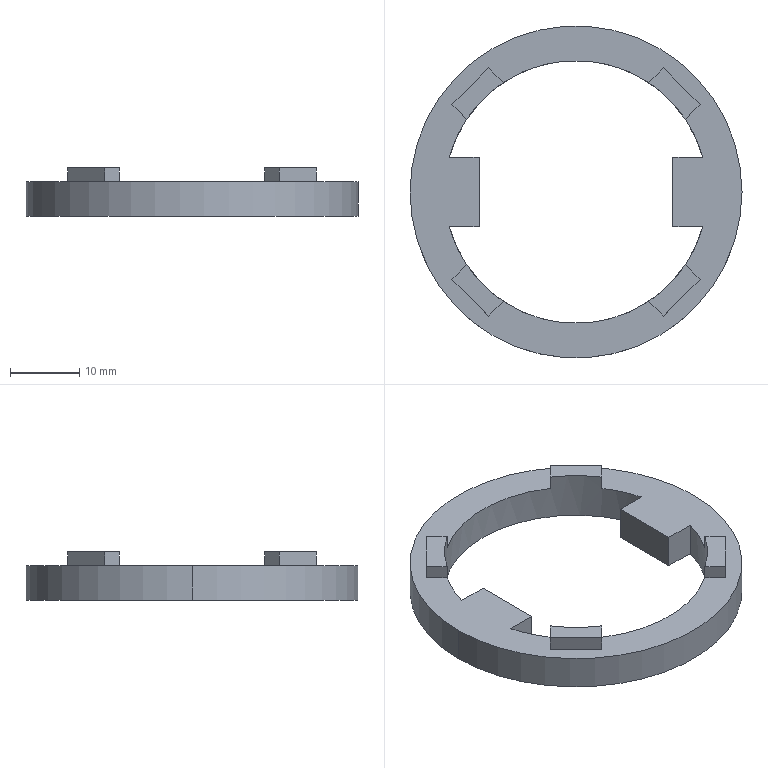Part | SolidWorks | features Extrusion 1, ICE 1 | 1 solid | 28 faces | box 48 x 48 x 7 mm | volume 4020 mm3 | plane 24 | cylinder 4 | commonest cylinder face diameters 38 x2 48 x2
STEP:
#1=CARTESIAN_POINT('',(24.,0.,5.));
#2=VERTEX_POINT('',#1);
#3=CARTESIAN_POINT('',(-24.,0.,5.));
#4=VERTEX_POINT('',#3);
#5=CARTESIAN_POINT('',(0.,0.,5.));
#6=DIRECTION('',(0.,0.,1.));
#7=DIRECTION('',(1.,0.,0.));
#8=AXIS2_PLACEMENT_3D('',#5,#6,#7);
#9=CIRCLE('',#8,24.);
#10=EDGE_CURVE('',#2,#4,#9,.T.);
#11=ORIENTED_EDGE('',*,*,#10,.F.);
#12=CARTESIAN_POINT('',(24.,0.,0.));
#13=VERTEX_POINT('',#12);
#14=CARTESIAN_POINT('',(24.,0.,5.));
#15=DIRECTION('',(0.,0.,-1.));
#16=VECTOR('',#15,1000.);
#17=LINE('',#14,#16);
#18=EDGE_CURVE('',#2,#13,#17,.T.);
#19=ORIENTED_EDGE('',*,*,#18,.T.);
#20=CARTESIAN_POINT('',(-24.,0.,0.));
#21=VERTEX_POINT('',#20);
#22=CARTESIAN_POINT('',(0.,0.,0.));
#23=DIRECTION('',(0.,0.,1.));
#24=DIRECTION('',(1.,0.,0.));
#25=AXIS2_PLACEMENT_3D('',#22,#23,#24);
#26=CIRCLE('',#25,24.);
#27=EDGE_CURVE('',#13,#21,#26,.T.);
#28=ORIENTED_EDGE('',*,*,#27,.T.);
#29=CARTESIAN_POINT('',(-24.,0.,5.));
#30=DIRECTION('',(0.,0.,-1.));
#31=VECTOR('',#30,1000.);
#32=LINE('',#29,#31);
#33=EDGE_CURVE('',#4,#21,#32,.T.);
#34=ORIENTED_EDGE('',*,*,#33,.F.);
#35=EDGE_LOOP('',(#11,#19,#28,#34));
#36=FACE_OUTER_BOUND('',#35,.T.);
#37=CARTESIAN_POINT('',(0.,0.,5.));
#38=DIRECTION('',(0.,0.,-1.));
#39=DIRECTION('',(-1.,0.,0.));
#40=AXIS2_PLACEMENT_3D('',#37,#38,#39);
#41=CYLINDRICAL_SURFACE('',#40,24.);
#42=ADVANCED_FACE('',(#36),#41,.T.);
#43=CARTESIAN_POINT('',(0.,0.,5.));
#44=DIRECTION('',(0.,0.,1.));
#45=DIRECTION('',(1.,0.,0.));
#46=AXIS2_PLACEMENT_3D('',#43,#44,#45);
#47=CIRCLE('',#46,24.);
#48=EDGE_CURVE('',#4,#2,#47,.T.);
#49=ORIENTED_EDGE('',*,*,#48,.T.);
#50=ORIENTED_EDGE('',*,*,#10,.T.);
#51=EDGE_LOOP('',(#49,#50));
#52=FACE_OUTER_BOUND('',#51,.T.);
#53=CARTESIAN_POINT('',(-17.944,-12.64,5.));
#54=VERTEX_POINT('',#53);
#55=CARTESIAN_POINT('',(-12.64,-17.944,5.));
#56=VERTEX_POINT('',#55);
#57=CARTESIAN_POINT('',(-12.64,-17.944,5.));
#58=DIRECTION('',(0.7071,-0.7071,0.));
#59=VECTOR('',#58,1000.);
#60=LINE('',#57,#59);
#61=EDGE_CURVE('',#54,#56,#60,.T.);
#62=ORIENTED_EDGE('',*,*,#61,.F.);
#63=CARTESIAN_POINT('',(-15.822,-10.519,5.));
#64=VERTEX_POINT('',#63);
#65=CARTESIAN_POINT('',(-15.822,-10.519,5.));
#66=DIRECTION('',(-0.7071,-0.7071,0.));
#67=VECTOR('',#66,1000.);
#68=LINE('',#65,#67);
#69=EDGE_CURVE('',#64,#54,#68,.T.);
#70=ORIENTED_EDGE('',*,*,#69,.F.);
#71=CARTESIAN_POINT('',(-18.33,-5.,5.));
#72=VERTEX_POINT('',#71);
#73=CARTESIAN_POINT('',(0.,0.,5.));
#74=DIRECTION('',(0.,0.,1.));
#75=DIRECTION('',(1.,0.,0.));
#76=AXIS2_PLACEMENT_3D('',#73,#74,#75);
#77=CIRCLE('',#76,19.);
#78=EDGE_CURVE('',#72,#64,#77,.T.);
#79=ORIENTED_EDGE('',*,*,#78,.F.);
#80=CARTESIAN_POINT('',(-14.,-5.,5.));
#81=VERTEX_POINT('',#80);
#82=CARTESIAN_POINT('',(-18.33,-5.,5.));
#83=DIRECTION('',(-1.,0.,0.));
#84=VECTOR('',#83,1000.);
#85=LINE('',#82,#84);
#86=EDGE_CURVE('',#81,#72,#85,.T.);
#87=ORIENTED_EDGE('',*,*,#86,.F.);
#88=CARTESIAN_POINT('',(-14.,5.,5.));
#89=VERTEX_POINT('',#88);
#90=CARTESIAN_POINT('',(-14.,5.,5.));
#91=DIRECTION('',(0.,-1.,0.));
#92=VECTOR('',#91,1000.);
#93=LINE('',#90,#92);
#94=EDGE_CURVE('',#89,#81,#93,.T.);
#95=ORIENTED_EDGE('',*,*,#94,.F.);
#96=CARTESIAN_POINT('',(-18.33,5.,5.));
#97=VERTEX_POINT('',#96);
#98=CARTESIAN_POINT('',(-18.33,5.,5.));
#99=DIRECTION('',(1.,0.,0.));
#100=VECTOR('',#99,1000.);
#101=LINE('',#98,#100);
#102=EDGE_CURVE('',#97,#89,#101,.T.);
#103=ORIENTED_EDGE('',*,*,#102,.F.);
#104=CARTESIAN_POINT('',(-15.822,10.519,5.));
#105=VERTEX_POINT('',#104);
#106=CARTESIAN_POINT('',(0.,0.,5.));
#107=DIRECTION('',(0.,0.,1.));
#108=DIRECTION('',(1.,0.,0.));
#109=AXIS2_PLACEMENT_3D('',#106,#107,#108);
#110=CIRCLE('',#109,19.);
#111=EDGE_CURVE('',#105,#97,#110,.T.);
#112=ORIENTED_EDGE('',*,*,#111,.F.);
#113=CARTESIAN_POINT('',(-17.944,12.64,5.));
#114=VERTEX_POINT('',#113);
#115=CARTESIAN_POINT('',(-15.822,10.519,5.));
#116=DIRECTION('',(0.7071,-0.7071,0.));
#117=VECTOR('',#116,1000.);
#118=LINE('',#115,#117);
#119=EDGE_CURVE('',#114,#105,#118,.T.);
#120=ORIENTED_EDGE('',*,*,#119,.F.);
#121=CARTESIAN_POINT('',(-12.64,17.944,5.));
#122=VERTEX_POINT('',#121);
#123=CARTESIAN_POINT('',(-17.944,12.64,5.));
#124=DIRECTION('',(-0.7071,-0.7071,0.));
#125=VECTOR('',#124,1000.);
#126=LINE('',#123,#125);
#127=EDGE_CURVE('',#122,#114,#126,.T.);
#128=ORIENTED_EDGE('',*,*,#127,.F.);
#129=CARTESIAN_POINT('',(-10.519,15.822,5.));
#130=VERTEX_POINT('',#129);
#131=CARTESIAN_POINT('',(-10.519,15.822,5.));
#132=DIRECTION('',(-0.7071,0.7071,0.));
#133=VECTOR('',#132,1000.);
#134=LINE('',#131,#133);
#135=EDGE_CURVE('',#130,#122,#134,.T.);
#136=ORIENTED_EDGE('',*,*,#135,.F.);
#137=CARTESIAN_POINT('',(10.519,15.822,5.));
#138=VERTEX_POINT('',#137);
#139=CARTESIAN_POINT('',(0.,0.,5.));
#140=DIRECTION('',(0.,0.,1.));
#141=DIRECTION('',(1.,0.,0.));
#142=AXIS2_PLACEMENT_3D('',#139,#140,#141);
#143=CIRCLE('',#142,19.);
#144=EDGE_CURVE('',#138,#130,#143,.T.);
#145=ORIENTED_EDGE('',*,*,#144,.F.);
#146=CARTESIAN_POINT('',(12.64,17.944,5.));
#147=VERTEX_POINT('',#146);
#148=CARTESIAN_POINT('',(10.519,15.822,5.));
#149=DIRECTION('',(-0.7071,-0.7071,0.));
#150=VECTOR('',#149,1000.);
#151=LINE('',#148,#150);
#152=EDGE_CURVE('',#147,#138,#151,.T.);
#153=ORIENTED_EDGE('',*,*,#152,.F.);
#154=CARTESIAN_POINT('',(17.944,12.64,5.));
#155=VERTEX_POINT('',#154);
#156=CARTESIAN_POINT('',(12.64,17.944,5.));
#157=DIRECTION('',(-0.7071,0.7071,0.));
#158=VECTOR('',#157,1000.);
#159=LINE('',#156,#158);
#160=EDGE_CURVE('',#155,#147,#159,.T.);
#161=ORIENTED_EDGE('',*,*,#160,.F.);
#162=CARTESIAN_POINT('',(15.822,10.519,5.));
#163=VERTEX_POINT('',#162);
#164=CARTESIAN_POINT('',(15.822,10.519,5.));
#165=DIRECTION('',(0.7071,0.7071,0.));
#166=VECTOR('',#165,1000.);
#167=LINE('',#164,#166);
#168=EDGE_CURVE('',#163,#155,#167,.T.);
#169=ORIENTED_EDGE('',*,*,#168,.F.);
#170=CARTESIAN_POINT('',(18.33,5.,5.));
#171=VERTEX_POINT('',#170);
#172=CARTESIAN_POINT('',(0.,0.,5.));
#173=DIRECTION('',(0.,0.,1.));
#174=DIRECTION('',(1.,0.,0.));
#175=AXIS2_PLACEMENT_3D('',#172,#173,#174);
#176=CIRCLE('',#175,19.);
#177=EDGE_CURVE('',#171,#163,#176,.T.);
#178=ORIENTED_EDGE('',*,*,#177,.F.);
#179=CARTESIAN_POINT('',(14.,5.,5.));
#180=VERTEX_POINT('',#179);
#181=CARTESIAN_POINT('',(18.33,5.,5.));
#182=DIRECTION('',(1.,0.,0.));
#183=VECTOR('',#182,1000.);
#184=LINE('',#181,#183);
#185=EDGE_CURVE('',#180,#171,#184,.T.);
#186=ORIENTED_EDGE('',*,*,#185,.F.);
#187=CARTESIAN_POINT('',(14.,-5.,5.));
#188=VERTEX_POINT('',#187);
#189=CARTESIAN_POINT('',(14.,5.,5.));
#190=DIRECTION('',(0.,1.,0.));
#191=VECTOR('',#190,1000.);
#192=LINE('',#189,#191);
#193=EDGE_CURVE('',#188,#180,#192,.T.);
#194=ORIENTED_EDGE('',*,*,#193,.F.);
#195=CARTESIAN_POINT('',(18.33,-5.,5.));
#196=VERTEX_POINT('',#195);
#197=CARTESIAN_POINT('',(18.33,-5.,5.));
#198=DIRECTION('',(-1.,0.,0.));
#199=VECTOR('',#198,1000.);
#200=LINE('',#197,#199);
#201=EDGE_CURVE('',#196,#188,#200,.T.);
#202=ORIENTED_EDGE('',*,*,#201,.F.);
#203=CARTESIAN_POINT('',(15.822,-10.519,5.));
#204=VERTEX_POINT('',#203);
#205=CARTESIAN_POINT('',(0.,0.,5.));
#206=DIRECTION('',(0.,0.,1.));
#207=DIRECTION('',(1.,0.,0.));
#208=AXIS2_PLACEMENT_3D('',#205,#206,#207);
#209=CIRCLE('',#208,19.);
#210=EDGE_CURVE('',#204,#196,#209,.T.);
#211=ORIENTED_EDGE('',*,*,#210,.F.);
#212=CARTESIAN_POINT('',(17.944,-12.64,5.));
#213=VERTEX_POINT('',#212);
#214=CARTESIAN_POINT('',(15.822,-10.519,5.));
#215=DIRECTION('',(-0.7071,0.7071,0.));
#216=VECTOR('',#215,1000.);
#217=LINE('',#214,#216);
#218=EDGE_CURVE('',#213,#204,#217,.T.);
#219=ORIENTED_EDGE('',*,*,#218,.F.);
#220=CARTESIAN_POINT('',(12.64,-17.944,5.));
#221=VERTEX_POINT('',#220);
#222=CARTESIAN_POINT('',(17.944,-12.64,5.));
#223=DIRECTION('',(0.7071,0.7071,0.));
#224=VECTOR('',#223,1000.);
#225=LINE('',#222,#224);
#226=EDGE_CURVE('',#221,#213,#225,.T.);
#227=ORIENTED_EDGE('',*,*,#226,.F.);
#228=CARTESIAN_POINT('',(10.519,-15.822,5.));
#229=VERTEX_POINT('',#228);
#230=CARTESIAN_POINT('',(10.519,-15.822,5.));
#231=DIRECTION('',(0.7071,-0.7071,0.));
#232=VECTOR('',#231,1000.);
#233=LINE('',#230,#232);
#234=EDGE_CURVE('',#229,#221,#233,.T.);
#235=ORIENTED_EDGE('',*,*,#234,.F.);
#236=CARTESIAN_POINT('',(-10.519,-15.822,5.));
#237=VERTEX_POINT('',#236);
#238=CARTESIAN_POINT('',(0.,0.,5.));
#239=DIRECTION('',(0.,0.,1.));
#240=DIRECTION('',(1.,0.,0.));
#241=AXIS2_PLACEMENT_3D('',#238,#239,#240);
#242=CIRCLE('',#241,19.);
#243=EDGE_CURVE('',#237,#229,#242,.T.);
#244=ORIENTED_EDGE('',*,*,#243,.F.);
#245=CARTESIAN_POINT('',(-10.519,-15.822,5.));
#246=DIRECTION('',(0.7071,0.7071,0.));
#247=VECTOR('',#246,1000.);
#248=LINE('',#245,#247);
#249=EDGE_CURVE('',#56,#237,#248,.T.);
#250=ORIENTED_EDGE('',*,*,#249,.F.);
#251=EDGE_LOOP('',(#62,#70,#79,#87,#95,#103,#112,#120,#128,#136,#145,#153,#161,#169,#178,#186,#194,#202,#211,#219,#227,#235,#244,#250));
#252=FACE_BOUND('',#251,.T.);
#253=CARTESIAN_POINT('',(0.,0.,5.));
#254=DIRECTION('',(0.,0.,1.));
#255=DIRECTION('',(1.,0.,0.));
#256=AXIS2_PLACEMENT_3D('',#253,#254,#255);
#257=PLANE('',#256);
#258=ADVANCED_FACE('',(#52,#252),#257,.T.);
#259=CARTESIAN_POINT('',(0.,0.,0.));
#260=DIRECTION('',(0.,0.,1.));
#261=DIRECTION('',(1.,0.,0.));
#262=AXIS2_PLACEMENT_3D('',#259,#260,#261);
#263=CIRCLE('',#262,24.);
#264=EDGE_CURVE('',#21,#13,#263,.T.);
#265=ORIENTED_EDGE('',*,*,#264,.F.);
#266=ORIENTED_EDGE('',*,*,#27,.F.);
#267=EDGE_LOOP('',(#265,#266));
#268=FACE_OUTER_BOUND('',#267,.T.);
#269=CARTESIAN_POINT('',(18.33,5.,0.));
#270=VERTEX_POINT('',#269);
#271=CARTESIAN_POINT('',(-18.33,5.,0.));
#272=VERTEX_POINT('',#271);
#273=CARTESIAN_POINT('',(0.,0.,0.));
#274=DIRECTION('',(0.,0.,1.));
#275=DIRECTION('',(1.,0.,0.));
#276=AXIS2_PLACEMENT_3D('',#273,#274,#275);
#277=CIRCLE('',#276,19.);
#278=EDGE_CURVE('',#270,#272,#277,.T.);
#279=ORIENTED_EDGE('',*,*,#278,.T.);
#280=CARTESIAN_POINT('',(-14.,5.,0.));
#281=VERTEX_POINT('',#280);
#282=CARTESIAN_POINT('',(-18.33,5.,0.));
#283=DIRECTION('',(1.,0.,0.));
#284=VECTOR('',#283,1000.);
#285=LINE('',#282,#284);
#286=EDGE_CURVE('',#272,#281,#285,.T.);
#287=ORIENTED_EDGE('',*,*,#286,.T.);
#288=CARTESIAN_POINT('',(-14.,-5.,0.));
#289=VERTEX_POINT('',#288);
#290=CARTESIAN_POINT('',(-14.,5.,0.));
#291=DIRECTION('',(0.,-1.,0.));
#292=VECTOR('',#291,1000.);
#293=LINE('',#290,#292);
#294=EDGE_CURVE('',#281,#289,#293,.T.);
#295=ORIENTED_EDGE('',*,*,#294,.T.);
#296=CARTESIAN_POINT('',(-18.33,-5.,0.));
#297=VERTEX_POINT('',#296);
#298=CARTESIAN_POINT('',(-18.33,-5.,0.));
#299=DIRECTION('',(-1.,0.,0.));
#300=VECTOR('',#299,1000.);
#301=LINE('',#298,#300);
#302=EDGE_CURVE('',#289,#297,#301,.T.);
#303=ORIENTED_EDGE('',*,*,#302,.T.);
#304=CARTESIAN_POINT('',(18.33,-5.,0.));
#305=VERTEX_POINT('',#304);
#306=CARTESIAN_POINT('',(0.,0.,0.));
#307=DIRECTION('',(0.,0.,1.));
#308=DIRECTION('',(1.,0.,0.));
#309=AXIS2_PLACEMENT_3D('',#306,#307,#308);
#310=CIRCLE('',#309,19.);
#311=EDGE_CURVE('',#297,#305,#310,.T.);
#312=ORIENTED_EDGE('',*,*,#311,.T.);
#313=CARTESIAN_POINT('',(14.,-5.,0.));
#314=VERTEX_POINT('',#313);
#315=CARTESIAN_POINT('',(18.33,-5.,0.));
#316=DIRECTION('',(-1.,0.,0.));
#317=VECTOR('',#316,1000.);
#318=LINE('',#315,#317);
#319=EDGE_CURVE('',#305,#314,#318,.T.);
#320=ORIENTED_EDGE('',*,*,#319,.T.);
#321=CARTESIAN_POINT('',(14.,5.,0.));
#322=VERTEX_POINT('',#321);
#323=CARTESIAN_POINT('',(14.,5.,0.));
#324=DIRECTION('',(0.,1.,0.));
#325=VECTOR('',#324,1000.);
#326=LINE('',#323,#325);
#327=EDGE_CURVE('',#314,#322,#326,.T.);
#328=ORIENTED_EDGE('',*,*,#327,.T.);
#329=CARTESIAN_POINT('',(18.33,5.,0.));
#330=DIRECTION('',(1.,0.,0.));
#331=VECTOR('',#330,1000.);
#332=LINE('',#329,#331);
#333=EDGE_CURVE('',#322,#270,#332,.T.);
#334=ORIENTED_EDGE('',*,*,#333,.T.);
#335=EDGE_LOOP('',(#279,#287,#295,#303,#312,#320,#328,#334));
#336=FACE_BOUND('',#335,.T.);
#337=CARTESIAN_POINT('',(0.,0.,0.));
#338=DIRECTION('',(0.,0.,1.));
#339=DIRECTION('',(1.,0.,0.));
#340=AXIS2_PLACEMENT_3D('',#337,#338,#339);
#341=PLANE('',#340);
#342=ADVANCED_FACE('',(#268,#336),#341,.F.);
#343=ORIENTED_EDGE('',*,*,#18,.F.);
#344=ORIENTED_EDGE('',*,*,#48,.F.);
#345=ORIENTED_EDGE('',*,*,#33,.T.);
#346=ORIENTED_EDGE('',*,*,#264,.T.);
#347=EDGE_LOOP('',(#343,#344,#345,#346));
#348=FACE_OUTER_BOUND('',#347,.T.);
#349=CARTESIAN_POINT('',(0.,0.,5.));
#350=DIRECTION('',(0.,0.,-1.));
#351=DIRECTION('',(-1.,0.,0.));
#352=AXIS2_PLACEMENT_3D('',#349,#350,#351);
#353=CYLINDRICAL_SURFACE('',#352,24.);
#354=ADVANCED_FACE('',(#348),#353,.T.);
#355=ORIENTED_EDGE('',*,*,#278,.F.);
#356=CARTESIAN_POINT('',(18.33,5.,5.));
#357=DIRECTION('',(0.,0.,-1.));
#358=VECTOR('',#357,1000.);
#359=LINE('',#356,#358);
#360=EDGE_CURVE('',#171,#270,#359,.T.);
#361=ORIENTED_EDGE('',*,*,#360,.F.);
#362=ORIENTED_EDGE('',*,*,#177,.T.);
#363=CARTESIAN_POINT('',(15.822,10.519,7.));
#364=VERTEX_POINT('',#363);
#365=CARTESIAN_POINT('',(15.822,10.519,7.));
#366=DIRECTION('',(0.,0.,-1.));
#367=VECTOR('',#366,1000.);
#368=LINE('',#365,#367);
#369=EDGE_CURVE('',#364,#163,#368,.T.);
#370=ORIENTED_EDGE('',*,*,#369,.F.);
#371=CARTESIAN_POINT('',(10.519,15.822,7.));
#372=VERTEX_POINT('',#371);
#373=CARTESIAN_POINT('',(0.,0.,7.));
#374=DIRECTION('',(0.,0.,-1.));
#375=DIRECTION('',(1.,0.,0.));
#376=AXIS2_PLACEMENT_3D('',#373,#374,#375);
#377=CIRCLE('',#376,19.);
#378=EDGE_CURVE('',#372,#364,#377,.T.);
#379=ORIENTED_EDGE('',*,*,#378,.F.);
#380=CARTESIAN_POINT('',(10.519,15.822,7.));
#381=DIRECTION('',(0.,0.,-1.));
#382=VECTOR('',#381,1000.);
#383=LINE('',#380,#382);
#384=EDGE_CURVE('',#372,#138,#383,.T.);
#385=ORIENTED_EDGE('',*,*,#384,.T.);
#386=ORIENTED_EDGE('',*,*,#144,.T.);
#387=CARTESIAN_POINT('',(-10.519,15.822,7.));
#388=VERTEX_POINT('',#387);
#389=CARTESIAN_POINT('',(-10.519,15.822,7.));
#390=DIRECTION('',(0.,0.,-1.));
#391=VECTOR('',#390,1000.);
#392=LINE('',#389,#391);
#393=EDGE_CURVE('',#388,#130,#392,.T.);
#394=ORIENTED_EDGE('',*,*,#393,.F.);
#395=CARTESIAN_POINT('',(-15.822,10.519,7.));
#396=VERTEX_POINT('',#395);
#397=CARTESIAN_POINT('',(0.,0.,7.));
#398=DIRECTION('',(0.,0.,-1.));
#399=DIRECTION('',(1.,0.,0.));
#400=AXIS2_PLACEMENT_3D('',#397,#398,#399);
#401=CIRCLE('',#400,19.);
#402=EDGE_CURVE('',#396,#388,#401,.T.);
#403=ORIENTED_EDGE('',*,*,#402,.F.);
#404=CARTESIAN_POINT('',(-15.822,10.519,7.));
#405=DIRECTION('',(0.,0.,-1.));
#406=VECTOR('',#405,1000.);
#407=LINE('',#404,#406);
#408=EDGE_CURVE('',#396,#105,#407,.T.);
#409=ORIENTED_EDGE('',*,*,#408,.T.);
#410=ORIENTED_EDGE('',*,*,#111,.T.);
#411=CARTESIAN_POINT('',(-18.33,5.,5.));
#412=DIRECTION('',(0.,0.,-1.));
#413=VECTOR('',#412,1000.);
#414=LINE('',#411,#413);
#415=EDGE_CURVE('',#97,#272,#414,.T.);
#416=ORIENTED_EDGE('',*,*,#415,.T.);
#417=EDGE_LOOP('',(#355,#361,#362,#370,#379,#385,#386,#394,#403,#409,#410,#416));
#418=FACE_OUTER_BOUND('',#417,.T.);
#419=CARTESIAN_POINT('',(0.,0.,5.));
#420=DIRECTION('',(0.,0.,-1.));
#421=DIRECTION('',(-1.,0.,0.));
#422=AXIS2_PLACEMENT_3D('',#419,#420,#421);
#423=CYLINDRICAL_SURFACE('',#422,19.);
#424=ADVANCED_FACE('',(#418),#423,.F.);
#425=ORIENTED_EDGE('',*,*,#286,.F.);
#426=ORIENTED_EDGE('',*,*,#415,.F.);
#427=ORIENTED_EDGE('',*,*,#102,.T.);
#428=CARTESIAN_POINT('',(-14.,5.,5.));
#429=DIRECTION('',(0.,0.,-1.));
#430=VECTOR('',#429,1000.);
#431=LINE('',#428,#430);
#432=EDGE_CURVE('',#89,#281,#431,.T.);
#433=ORIENTED_EDGE('',*,*,#432,.T.);
#434=EDGE_LOOP('',(#425,#426,#427,#433));
#435=FACE_OUTER_BOUND('',#434,.T.);
#436=CARTESIAN_POINT('',(-18.33,5.,5.));
#437=DIRECTION('',(0.,1.,0.));
#438=DIRECTION('',(-1.,0.,0.));
#439=AXIS2_PLACEMENT_3D('',#436,#437,#438);
#440=PLANE('',#439);
#441=ADVANCED_FACE('',(#435),#440,.T.);
#442=ORIENTED_EDGE('',*,*,#294,.F.);
#443=ORIENTED_EDGE('',*,*,#432,.F.);
#444=ORIENTED_EDGE('',*,*,#94,.T.);
#445=CARTESIAN_POINT('',(-14.,-5.,5.));
#446=DIRECTION('',(0.,0.,-1.));
#447=VECTOR('',#446,1000.);
#448=LINE('',#445,#447);
#449=EDGE_CURVE('',#81,#289,#448,.T.);
#450=ORIENTED_EDGE('',*,*,#449,.T.);
#451=EDGE_LOOP('',(#442,#443,#444,#450));
#452=FACE_OUTER_BOUND('',#451,.T.);
#453=CARTESIAN_POINT('',(-14.,5.,5.));
#454=DIRECTION('',(1.,0.,0.));
#455=DIRECTION('',(0.,0.,-1.));
#456=AXIS2_PLACEMENT_3D('',#453,#454,#455);
#457=PLANE('',#456);
#458=ADVANCED_FACE('',(#452),#457,.T.);
#459=ORIENTED_EDGE('',*,*,#302,.F.);
#460=ORIENTED_EDGE('',*,*,#449,.F.);
#461=ORIENTED_EDGE('',*,*,#86,.T.);
#462=CARTESIAN_POINT('',(-18.33,-5.,5.));
#463=DIRECTION('',(0.,0.,-1.));
#464=VECTOR('',#463,1000.);
#465=LINE('',#462,#464);
#466=EDGE_CURVE('',#72,#297,#465,.T.);
#467=ORIENTED_EDGE('',*,*,#466,.T.);
#468=EDGE_LOOP('',(#459,#460,#461,#467));
#469=FACE_OUTER_BOUND('',#468,.T.);
#470=CARTESIAN_POINT('',(-18.33,-5.,5.));
#471=DIRECTION('',(0.,-1.,0.));
#472=DIRECTION('',(1.,0.,0.));
#473=AXIS2_PLACEMENT_3D('',#470,#471,#472);
#474=PLANE('',#473);
#475=ADVANCED_FACE('',(#469),#474,.T.);
#476=ORIENTED_EDGE('',*,*,#311,.F.);
#477=ORIENTED_EDGE('',*,*,#466,.F.);
#478=ORIENTED_EDGE('',*,*,#78,.T.);
#479=CARTESIAN_POINT('',(-15.822,-10.519,7.));
#480=VERTEX_POINT('',#479);
#481=CARTESIAN_POINT('',(-15.822,-10.519,7.));
#482=DIRECTION('',(0.,0.,-1.));
#483=VECTOR('',#482,1000.);
#484=LINE('',#481,#483);
#485=EDGE_CURVE('',#480,#64,#484,.T.);
#486=ORIENTED_EDGE('',*,*,#485,.F.);
#487=CARTESIAN_POINT('',(-10.519,-15.822,7.));
#488=VERTEX_POINT('',#487);
#489=CARTESIAN_POINT('',(0.,0.,7.));
#490=DIRECTION('',(0.,0.,-1.));
#491=DIRECTION('',(1.,0.,0.));
#492=AXIS2_PLACEMENT_3D('',#489,#490,#491);
#493=CIRCLE('',#492,19.);
#494=EDGE_CURVE('',#488,#480,#493,.T.);
#495=ORIENTED_EDGE('',*,*,#494,.F.);
#496=CARTESIAN_POINT('',(-10.519,-15.822,7.));
#497=DIRECTION('',(0.,0.,-1.));
#498=VECTOR('',#497,1000.);
#499=LINE('',#496,#498);
#500=EDGE_CURVE('',#488,#237,#499,.T.);
#501=ORIENTED_EDGE('',*,*,#500,.T.);
#502=ORIENTED_EDGE('',*,*,#243,.T.);
#503=CARTESIAN_POINT('',(10.519,-15.822,7.));
#504=VERTEX_POINT('',#503);
#505=CARTESIAN_POINT('',(10.519,-15.822,7.));
#506=DIRECTION('',(0.,0.,-1.));
#507=VECTOR('',#506,1000.);
#508=LINE('',#505,#507);
#509=EDGE_CURVE('',#504,#229,#508,.T.);
#510=ORIENTED_EDGE('',*,*,#509,.F.);
#511=CARTESIAN_POINT('',(15.822,-10.519,7.));
#512=VERTEX_POINT('',#511);
#513=CARTESIAN_POINT('',(0.,0.,7.));
#514=DIRECTION('',(0.,0.,-1.));
#515=DIRECTION('',(1.,0.,0.));
#516=AXIS2_PLACEMENT_3D('',#513,#514,#515);
#517=CIRCLE('',#516,19.);
#518=EDGE_CURVE('',#512,#504,#517,.T.);
#519=ORIENTED_EDGE('',*,*,#518,.F.);
#520=CARTESIAN_POINT('',(15.822,-10.519,7.));
#521=DIRECTION('',(0.,0.,-1.));
#522=VECTOR('',#521,1000.);
#523=LINE('',#520,#522);
#524=EDGE_CURVE('',#512,#204,#523,.T.);
#525=ORIENTED_EDGE('',*,*,#524,.T.);
#526=ORIENTED_EDGE('',*,*,#210,.T.);
#527=CARTESIAN_POINT('',(18.33,-5.,5.));
#528=DIRECTION('',(0.,0.,-1.));
#529=VECTOR('',#528,1000.);
#530=LINE('',#527,#529);
#531=EDGE_CURVE('',#196,#305,#530,.T.);
#532=ORIENTED_EDGE('',*,*,#531,.T.);
#533=EDGE_LOOP('',(#476,#477,#478,#486,#495,#501,#502,#510,#519,#525,#526,#532));
#534=FACE_OUTER_BOUND('',#533,.T.);
#535=CARTESIAN_POINT('',(0.,0.,5.));
#536=DIRECTION('',(0.,0.,-1.));
#537=DIRECTION('',(-1.,0.,0.));
#538=AXIS2_PLACEMENT_3D('',#535,#536,#537);
#539=CYLINDRICAL_SURFACE('',#538,19.);
#540=ADVANCED_FACE('',(#534),#539,.F.);
#541=ORIENTED_EDGE('',*,*,#319,.F.);
#542=ORIENTED_EDGE('',*,*,#531,.F.);
#543=ORIENTED_EDGE('',*,*,#201,.T.);
#544=CARTESIAN_POINT('',(14.,-5.,5.));
#545=DIRECTION('',(0.,0.,-1.));
#546=VECTOR('',#545,1000.);
#547=LINE('',#544,#546);
#548=EDGE_CURVE('',#188,#314,#547,.T.);
#549=ORIENTED_EDGE('',*,*,#548,.T.);
#550=EDGE_LOOP('',(#541,#542,#543,#549));
#551=FACE_OUTER_BOUND('',#550,.T.);
#552=CARTESIAN_POINT('',(18.33,-5.,5.));
#553=DIRECTION('',(0.,-1.,0.));
#554=DIRECTION('',(1.,0.,0.));
#555=AXIS2_PLACEMENT_3D('',#552,#553,#554);
#556=PLANE('',#555);
#557=ADVANCED_FACE('',(#551),#556,.T.);
#558=ORIENTED_EDGE('',*,*,#327,.F.);
#559=ORIENTED_EDGE('',*,*,#548,.F.);
#560=ORIENTED_EDGE('',*,*,#193,.T.);
#561=CARTESIAN_POINT('',(14.,5.,5.));
#562=DIRECTION('',(0.,0.,-1.));
#563=VECTOR('',#562,1000.);
#564=LINE('',#561,#563);
#565=EDGE_CURVE('',#180,#322,#564,.T.);
#566=ORIENTED_EDGE('',*,*,#565,.T.);
#567=EDGE_LOOP('',(#558,#559,#560,#566));
#568=FACE_OUTER_BOUND('',#567,.T.);
#569=CARTESIAN_POINT('',(14.,5.,5.));
#570=DIRECTION('',(-1.,0.,0.));
#571=DIRECTION('',(0.,0.,1.));
#572=AXIS2_PLACEMENT_3D('',#569,#570,#571);
#573=PLANE('',#572);
#574=ADVANCED_FACE('',(#568),#573,.T.);
#575=ORIENTED_EDGE('',*,*,#333,.F.);
#576=ORIENTED_EDGE('',*,*,#565,.F.);
#577=ORIENTED_EDGE('',*,*,#185,.T.);
#578=ORIENTED_EDGE('',*,*,#360,.T.);
#579=EDGE_LOOP('',(#575,#576,#577,#578));
#580=FACE_OUTER_BOUND('',#579,.T.);
#581=CARTESIAN_POINT('',(18.33,5.,5.));
#582=DIRECTION('',(0.,1.,0.));
#583=DIRECTION('',(-1.,0.,0.));
#584=AXIS2_PLACEMENT_3D('',#581,#582,#583);
#585=PLANE('',#584);
#586=ADVANCED_FACE('',(#580),#585,.T.);
#587=ORIENTED_EDGE('',*,*,#135,.T.);
#588=CARTESIAN_POINT('',(-12.64,17.944,7.));
#589=VERTEX_POINT('',#588);
#590=CARTESIAN_POINT('',(-12.64,17.944,7.));
#591=DIRECTION('',(0.,0.,-1.));
#592=VECTOR('',#591,1000.);
#593=LINE('',#590,#592);
#594=EDGE_CURVE('',#589,#122,#593,.T.);
#595=ORIENTED_EDGE('',*,*,#594,.F.);
#596=CARTESIAN_POINT('',(-10.519,15.822,7.));
#597=DIRECTION('',(-0.7071,0.7071,0.));
#598=VECTOR('',#597,1000.);
#599=LINE('',#596,#598);
#600=EDGE_CURVE('',#388,#589,#599,.T.);
#601=ORIENTED_EDGE('',*,*,#600,.F.);
#602=ORIENTED_EDGE('',*,*,#393,.T.);
#603=EDGE_LOOP('',(#587,#595,#601,#602));
#604=FACE_OUTER_BOUND('',#603,.T.);
#605=CARTESIAN_POINT('',(-10.519,15.822,7.));
#606=DIRECTION('',(-0.7071,-0.7071,0.));
#607=DIRECTION('',(0.7071,-0.7071,0.));
#608=AXIS2_PLACEMENT_3D('',#605,#606,#607);
#609=PLANE('',#608);
#610=ADVANCED_FACE('',(#604),#609,.F.);
#611=ORIENTED_EDGE('',*,*,#127,.T.);
#612=CARTESIAN_POINT('',(-17.944,12.64,7.));
#613=VERTEX_POINT('',#612);
#614=CARTESIAN_POINT('',(-17.944,12.64,7.));
#615=DIRECTION('',(0.,0.,-1.));
#616=VECTOR('',#615,1000.);
#617=LINE('',#614,#616);
#618=EDGE_CURVE('',#613,#114,#617,.T.);
#619=ORIENTED_EDGE('',*,*,#618,.F.);
#620=CARTESIAN_POINT('',(-17.944,12.64,7.));
#621=DIRECTION('',(-0.7071,-0.7071,0.));
#622=VECTOR('',#621,1000.);
#623=LINE('',#620,#622);
#624=EDGE_CURVE('',#589,#613,#623,.T.);
#625=ORIENTED_EDGE('',*,*,#624,.F.);
#626=ORIENTED_EDGE('',*,*,#594,.T.);
#627=EDGE_LOOP('',(#611,#619,#625,#626));
#628=FACE_OUTER_BOUND('',#627,.T.);
#629=CARTESIAN_POINT('',(-17.944,12.64,7.));
#630=DIRECTION('',(0.7071,-0.7071,0.));
#631=DIRECTION('',(0.7071,0.7071,0.));
#632=AXIS2_PLACEMENT_3D('',#629,#630,#631);
#633=PLANE('',#632);
#634=ADVANCED_FACE('',(#628),#633,.F.);
#635=ORIENTED_EDGE('',*,*,#119,.T.);
#636=ORIENTED_EDGE('',*,*,#408,.F.);
#637=CARTESIAN_POINT('',(-15.822,10.519,7.));
#638=DIRECTION('',(0.7071,-0.7071,0.));
#639=VECTOR('',#638,1000.);
#640=LINE('',#637,#639);
#641=EDGE_CURVE('',#613,#396,#640,.T.);
#642=ORIENTED_EDGE('',*,*,#641,.F.);
#643=ORIENTED_EDGE('',*,*,#618,.T.);
#644=EDGE_LOOP('',(#635,#636,#642,#643));
#645=FACE_OUTER_BOUND('',#644,.T.);
#646=CARTESIAN_POINT('',(-15.822,10.519,7.));
#647=DIRECTION('',(0.7071,0.7071,0.));
#648=DIRECTION('',(-0.7071,0.7071,0.));
#649=AXIS2_PLACEMENT_3D('',#646,#647,#648);
#650=PLANE('',#649);
#651=ADVANCED_FACE('',(#645),#650,.F.);
#652=ORIENTED_EDGE('',*,*,#402,.T.);
#653=ORIENTED_EDGE('',*,*,#600,.T.);
#654=ORIENTED_EDGE('',*,*,#624,.T.);
#655=ORIENTED_EDGE('',*,*,#641,.T.);
#656=EDGE_LOOP('',(#652,#653,#654,#655));
#657=FACE_OUTER_BOUND('',#656,.T.);
#658=CARTESIAN_POINT('',(0.,0.,7.));
#659=DIRECTION('',(0.,0.,1.));
#660=DIRECTION('',(1.,0.,0.));
#661=AXIS2_PLACEMENT_3D('',#658,#659,#660);
#662=PLANE('',#661);
#663=ADVANCED_FACE('',(#657),#662,.T.);
#664=ORIENTED_EDGE('',*,*,#168,.T.);
#665=CARTESIAN_POINT('',(17.944,12.64,7.));
#666=VERTEX_POINT('',#665);
#667=CARTESIAN_POINT('',(17.944,12.64,7.));
#668=DIRECTION('',(0.,0.,-1.));
#669=VECTOR('',#668,1000.);
#670=LINE('',#667,#669);
#671=EDGE_CURVE('',#666,#155,#670,.T.);
#672=ORIENTED_EDGE('',*,*,#671,.F.);
#673=CARTESIAN_POINT('',(15.822,10.519,7.));
#674=DIRECTION('',(0.7071,0.7071,0.));
#675=VECTOR('',#674,1000.);
#676=LINE('',#673,#675);
#677=EDGE_CURVE('',#364,#666,#676,.T.);
#678=ORIENTED_EDGE('',*,*,#677,.F.);
#679=ORIENTED_EDGE('',*,*,#369,.T.);
#680=EDGE_LOOP('',(#664,#672,#678,#679));
#681=FACE_OUTER_BOUND('',#680,.T.);
#682=CARTESIAN_POINT('',(15.822,10.519,7.));
#683=DIRECTION('',(-0.7071,0.7071,0.));
#684=DIRECTION('',(-0.7071,-0.7071,0.));
#685=AXIS2_PLACEMENT_3D('',#682,#683,#684);
#686=PLANE('',#685);
#687=ADVANCED_FACE('',(#681),#686,.F.);
#688=ORIENTED_EDGE('',*,*,#160,.T.);
#689=CARTESIAN_POINT('',(12.64,17.944,7.));
#690=VERTEX_POINT('',#689);
#691=CARTESIAN_POINT('',(12.64,17.944,7.));
#692=DIRECTION('',(0.,0.,-1.));
#693=VECTOR('',#692,1000.);
#694=LINE('',#691,#693);
#695=EDGE_CURVE('',#690,#147,#694,.T.);
#696=ORIENTED_EDGE('',*,*,#695,.F.);
#697=CARTESIAN_POINT('',(12.64,17.944,7.));
#698=DIRECTION('',(-0.7071,0.7071,0.));
#699=VECTOR('',#698,1000.);
#700=LINE('',#697,#699);
#701=EDGE_CURVE('',#666,#690,#700,.T.);
#702=ORIENTED_EDGE('',*,*,#701,.F.);
#703=ORIENTED_EDGE('',*,*,#671,.T.);
#704=EDGE_LOOP('',(#688,#696,#702,#703));
#705=FACE_OUTER_BOUND('',#704,.T.);
#706=CARTESIAN_POINT('',(12.64,17.944,7.));
#707=DIRECTION('',(-0.7071,-0.7071,0.));
#708=DIRECTION('',(0.7071,-0.7071,0.));
#709=AXIS2_PLACEMENT_3D('',#706,#707,#708);
#710=PLANE('',#709);
#711=ADVANCED_FACE('',(#705),#710,.F.);
#712=ORIENTED_EDGE('',*,*,#152,.T.);
#713=ORIENTED_EDGE('',*,*,#384,.F.);
#714=CARTESIAN_POINT('',(10.519,15.822,7.));
#715=DIRECTION('',(-0.7071,-0.7071,0.));
#716=VECTOR('',#715,1000.);
#717=LINE('',#714,#716);
#718=EDGE_CURVE('',#690,#372,#717,.T.);
#719=ORIENTED_EDGE('',*,*,#718,.F.);
#720=ORIENTED_EDGE('',*,*,#695,.T.);
#721=EDGE_LOOP('',(#712,#713,#719,#720));
#722=FACE_OUTER_BOUND('',#721,.T.);
#723=CARTESIAN_POINT('',(10.519,15.822,7.));
#724=DIRECTION('',(0.7071,-0.7071,0.));
#725=DIRECTION('',(0.7071,0.7071,0.));
#726=AXIS2_PLACEMENT_3D('',#723,#724,#725);
#727=PLANE('',#726);
#728=ADVANCED_FACE('',(#722),#727,.F.);
#729=ORIENTED_EDGE('',*,*,#378,.T.);
#730=ORIENTED_EDGE('',*,*,#677,.T.);
#731=ORIENTED_EDGE('',*,*,#701,.T.);
#732=ORIENTED_EDGE('',*,*,#718,.T.);
#733=EDGE_LOOP('',(#729,#730,#731,#732));
#734=FACE_OUTER_BOUND('',#733,.T.);
#735=CARTESIAN_POINT('',(0.,0.,7.));
#736=DIRECTION('',(0.,0.,1.));
#737=DIRECTION('',(1.,0.,0.));
#738=AXIS2_PLACEMENT_3D('',#735,#736,#737);
#739=PLANE('',#738);
#740=ADVANCED_FACE('',(#734),#739,.T.);
#741=ORIENTED_EDGE('',*,*,#234,.T.);
#742=CARTESIAN_POINT('',(12.64,-17.944,7.));
#743=VERTEX_POINT('',#742);
#744=CARTESIAN_POINT('',(12.64,-17.944,7.));
#745=DIRECTION('',(0.,0.,-1.));
#746=VECTOR('',#745,1000.);
#747=LINE('',#744,#746);
#748=EDGE_CURVE('',#743,#221,#747,.T.);
#749=ORIENTED_EDGE('',*,*,#748,.F.);
#750=CARTESIAN_POINT('',(10.519,-15.822,7.));
#751=DIRECTION('',(0.7071,-0.7071,0.));
#752=VECTOR('',#751,1000.);
#753=LINE('',#750,#752);
#754=EDGE_CURVE('',#504,#743,#753,.T.);
#755=ORIENTED_EDGE('',*,*,#754,.F.);
#756=ORIENTED_EDGE('',*,*,#509,.T.);
#757=EDGE_LOOP('',(#741,#749,#755,#756));
#758=FACE_OUTER_BOUND('',#757,.T.);
#759=CARTESIAN_POINT('',(10.519,-15.822,7.));
#760=DIRECTION('',(0.7071,0.7071,0.));
#761=DIRECTION('',(-0.7071,0.7071,0.));
#762=AXIS2_PLACEMENT_3D('',#759,#760,#761);
#763=PLANE('',#762);
#764=ADVANCED_FACE('',(#758),#763,.F.);
#765=ORIENTED_EDGE('',*,*,#226,.T.);
#766=CARTESIAN_POINT('',(17.944,-12.64,7.));
#767=VERTEX_POINT('',#766);
#768=CARTESIAN_POINT('',(17.944,-12.64,7.));
#769=DIRECTION('',(0.,0.,-1.));
#770=VECTOR('',#769,1000.);
#771=LINE('',#768,#770);
#772=EDGE_CURVE('',#767,#213,#771,.T.);
#773=ORIENTED_EDGE('',*,*,#772,.F.);
#774=CARTESIAN_POINT('',(17.944,-12.64,7.));
#775=DIRECTION('',(0.7071,0.7071,0.));
#776=VECTOR('',#775,1000.);
#777=LINE('',#774,#776);
#778=EDGE_CURVE('',#743,#767,#777,.T.);
#779=ORIENTED_EDGE('',*,*,#778,.F.);
#780=ORIENTED_EDGE('',*,*,#748,.T.);
#781=EDGE_LOOP('',(#765,#773,#779,#780));
#782=FACE_OUTER_BOUND('',#781,.T.);
#783=CARTESIAN_POINT('',(17.944,-12.64,7.));
#784=DIRECTION('',(-0.7071,0.7071,0.));
#785=DIRECTION('',(-0.7071,-0.7071,0.));
#786=AXIS2_PLACEMENT_3D('',#783,#784,#785);
#787=PLANE('',#786);
#788=ADVANCED_FACE('',(#782),#787,.F.);
#789=ORIENTED_EDGE('',*,*,#218,.T.);
#790=ORIENTED_EDGE('',*,*,#524,.F.);
#791=CARTESIAN_POINT('',(15.822,-10.519,7.));
#792=DIRECTION('',(-0.7071,0.7071,0.));
#793=VECTOR('',#792,1000.);
#794=LINE('',#791,#793);
#795=EDGE_CURVE('',#767,#512,#794,.T.);
#796=ORIENTED_EDGE('',*,*,#795,.F.);
#797=ORIENTED_EDGE('',*,*,#772,.T.);
#798=EDGE_LOOP('',(#789,#790,#796,#797));
#799=FACE_OUTER_BOUND('',#798,.T.);
#800=CARTESIAN_POINT('',(15.822,-10.519,7.));
#801=DIRECTION('',(-0.7071,-0.7071,0.));
#802=DIRECTION('',(0.7071,-0.7071,0.));
#803=AXIS2_PLACEMENT_3D('',#800,#801,#802);
#804=PLANE('',#803);
#805=ADVANCED_FACE('',(#799),#804,.F.);
#806=ORIENTED_EDGE('',*,*,#518,.T.);
#807=ORIENTED_EDGE('',*,*,#754,.T.);
#808=ORIENTED_EDGE('',*,*,#778,.T.);
#809=ORIENTED_EDGE('',*,*,#795,.T.);
#810=EDGE_LOOP('',(#806,#807,#808,#809));
#811=FACE_OUTER_BOUND('',#810,.T.);
#812=CARTESIAN_POINT('',(0.,0.,7.));
#813=DIRECTION('',(0.,0.,1.));
#814=DIRECTION('',(1.,0.,0.));
#815=AXIS2_PLACEMENT_3D('',#812,#813,#814);
#816=PLANE('',#815);
#817=ADVANCED_FACE('',(#811),#816,.T.);
#818=ORIENTED_EDGE('',*,*,#69,.T.);
#819=CARTESIAN_POINT('',(-17.944,-12.64,7.));
#820=VERTEX_POINT('',#819);
#821=CARTESIAN_POINT('',(-17.944,-12.64,7.));
#822=DIRECTION('',(0.,0.,-1.));
#823=VECTOR('',#822,1000.);
#824=LINE('',#821,#823);
#825=EDGE_CURVE('',#820,#54,#824,.T.);
#826=ORIENTED_EDGE('',*,*,#825,.F.);
#827=CARTESIAN_POINT('',(-15.822,-10.519,7.));
#828=DIRECTION('',(-0.7071,-0.7071,0.));
#829=VECTOR('',#828,1000.);
#830=LINE('',#827,#829);
#831=EDGE_CURVE('',#480,#820,#830,.T.);
#832=ORIENTED_EDGE('',*,*,#831,.F.);
#833=ORIENTED_EDGE('',*,*,#485,.T.);
#834=EDGE_LOOP('',(#818,#826,#832,#833));
#835=FACE_OUTER_BOUND('',#834,.T.);
#836=CARTESIAN_POINT('',(-15.822,-10.519,7.));
#837=DIRECTION('',(0.7071,-0.7071,0.));
#838=DIRECTION('',(0.7071,0.7071,0.));
#839=AXIS2_PLACEMENT_3D('',#836,#837,#838);
#840=PLANE('',#839);
#841=ADVANCED_FACE('',(#835),#840,.F.);
#842=ORIENTED_EDGE('',*,*,#61,.T.);
#843=CARTESIAN_POINT('',(-12.64,-17.944,7.));
#844=VERTEX_POINT('',#843);
#845=CARTESIAN_POINT('',(-12.64,-17.944,7.));
#846=DIRECTION('',(0.,0.,-1.));
#847=VECTOR('',#846,1000.);
#848=LINE('',#845,#847);
#849=EDGE_CURVE('',#844,#56,#848,.T.);
#850=ORIENTED_EDGE('',*,*,#849,.F.);
#851=CARTESIAN_POINT('',(-12.64,-17.944,7.));
#852=DIRECTION('',(0.7071,-0.7071,0.));
#853=VECTOR('',#852,1000.);
#854=LINE('',#851,#853);
#855=EDGE_CURVE('',#820,#844,#854,.T.);
#856=ORIENTED_EDGE('',*,*,#855,.F.);
#857=ORIENTED_EDGE('',*,*,#825,.T.);
#858=EDGE_LOOP('',(#842,#850,#856,#857));
#859=FACE_OUTER_BOUND('',#858,.T.);
#860=CARTESIAN_POINT('',(-12.64,-17.944,7.));
#861=DIRECTION('',(0.7071,0.7071,0.));
#862=DIRECTION('',(-0.7071,0.7071,0.));
#863=AXIS2_PLACEMENT_3D('',#860,#861,#862);
#864=PLANE('',#863);
#865=ADVANCED_FACE('',(#859),#864,.F.);
#866=ORIENTED_EDGE('',*,*,#249,.T.);
#867=ORIENTED_EDGE('',*,*,#500,.F.);
#868=CARTESIAN_POINT('',(-10.519,-15.822,7.));
#869=DIRECTION('',(0.7071,0.7071,0.));
#870=VECTOR('',#869,1000.);
#871=LINE('',#868,#870);
#872=EDGE_CURVE('',#844,#488,#871,.T.);
#873=ORIENTED_EDGE('',*,*,#872,.F.);
#874=ORIENTED_EDGE('',*,*,#849,.T.);
#875=EDGE_LOOP('',(#866,#867,#873,#874));
#876=FACE_OUTER_BOUND('',#875,.T.);
#877=CARTESIAN_POINT('',(-10.519,-15.822,7.));
#878=DIRECTION('',(-0.7071,0.7071,0.));
#879=DIRECTION('',(-0.7071,-0.7071,0.));
#880=AXIS2_PLACEMENT_3D('',#877,#878,#879);
#881=PLANE('',#880);
#882=ADVANCED_FACE('',(#876),#881,.F.);
#883=ORIENTED_EDGE('',*,*,#494,.T.);
#884=ORIENTED_EDGE('',*,*,#831,.T.);
#885=ORIENTED_EDGE('',*,*,#855,.T.);
#886=ORIENTED_EDGE('',*,*,#872,.T.);
#887=EDGE_LOOP('',(#883,#884,#885,#886));
#888=FACE_OUTER_BOUND('',#887,.T.);
#889=CARTESIAN_POINT('',(0.,0.,7.));
#890=DIRECTION('',(0.,0.,1.));
#891=DIRECTION('',(1.,0.,0.));
#892=AXIS2_PLACEMENT_3D('',#889,#890,#891);
#893=PLANE('',#892);
#894=ADVANCED_FACE('',(#888),#893,.T.);
#895=CLOSED_SHELL('',(#42,#258,#342,#354,#424,#441,#458,#475,#540,#557,#574,#586,#610,#634,#651,#663,#687,#711,#728,#740,#764,#788,#805,#817,#841,#865,#882,#894));
#896=MANIFOLD_SOLID_BREP('',#895);
#897=CARTESIAN_POINT('',(0.,0.,0.));
#898=DIRECTION('',(0.,0.,1.));
#899=DIRECTION('',(1.,0.,0.));
#900=AXIS2_PLACEMENT_3D('',#897,#898,#899);
#901=(LENGTH_UNIT()NAMED_UNIT(*)SI_UNIT(.MILLI.,.METRE.));
#902=UNCERTAINTY_MEASURE_WITH_UNIT(LENGTH_MEASURE(0.00001),#901,'','');
#903=(NAMED_UNIT(*)PLANE_ANGLE_UNIT()SI_UNIT($,.RADIAN.));
#904=(NAMED_UNIT(*)SI_UNIT($,.STERADIAN.)SOLID_ANGLE_UNIT());
#905=(GEOMETRIC_REPRESENTATION_CONTEXT(3)GLOBAL_UNCERTAINTY_ASSIGNED_CONTEXT((#902))GLOBAL_UNIT_ASSIGNED_CONTEXT((#901,#903,#904))REPRESENTATION_CONTEXT('',''));
#906=ADVANCED_BREP_SHAPE_REPRESENTATION('',(#896,#900),#905);